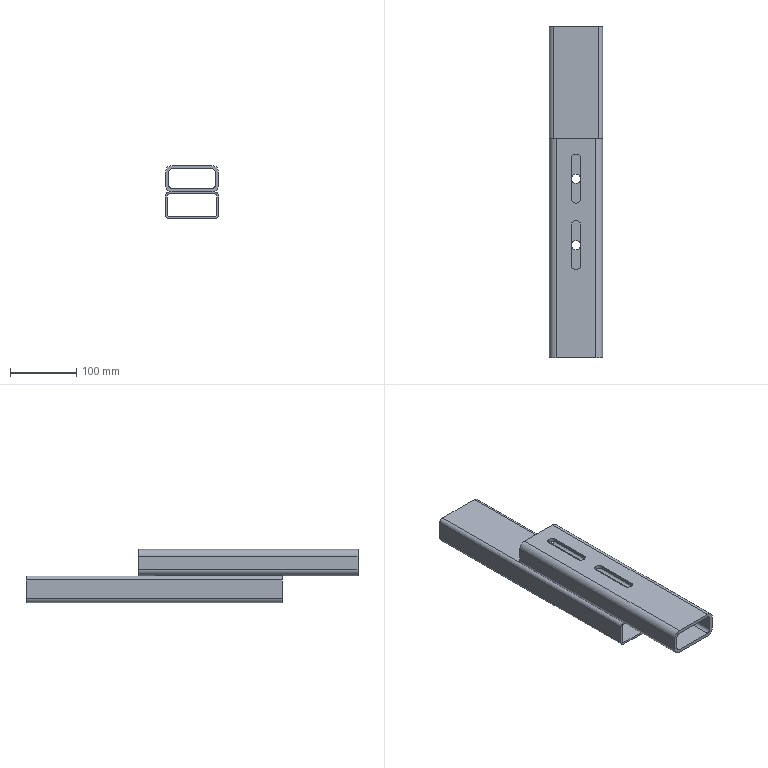Part | STEP file | rectangular upper-left | 2 solids | 56 faces | box 80 x 500 x 80 mm | volume 574998 mm3 | plane 28 | cylinder 28 | commonest cylinder face diameters 14 x12 6 x4 10 x4 12 x4 20 x4